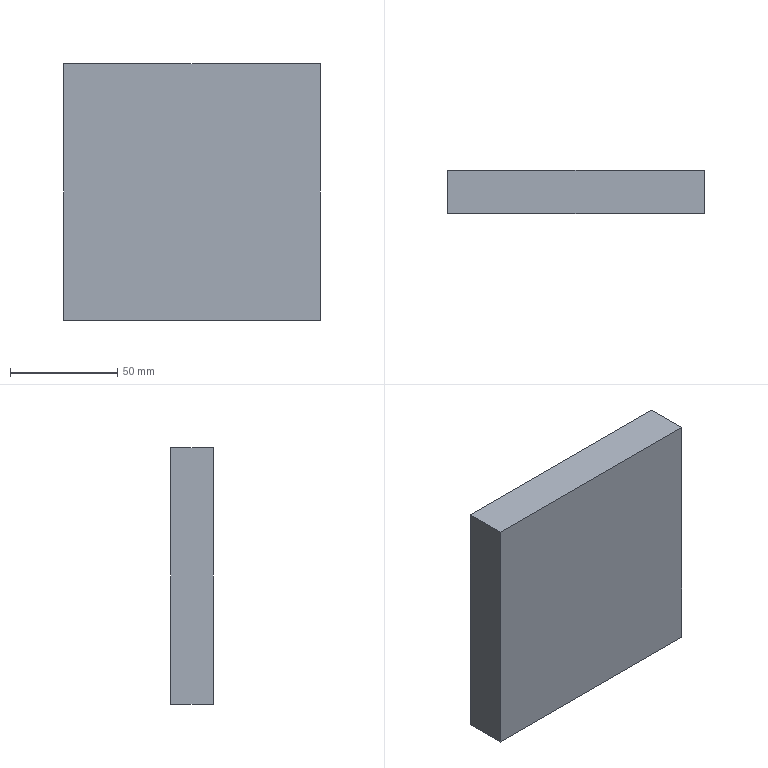Part | SolidWorks | features Extrusion 1 | 1 solid | 6 faces | box 120 x 20 x 120 mm | volume 288000 mm3 | plane 6
STEP:
#1=CARTESIAN_POINT('',(60.,0.,60.));
#2=VERTEX_POINT('',#1);
#3=CARTESIAN_POINT('',(60.,0.,-60.));
#4=VERTEX_POINT('',#3);
#5=CARTESIAN_POINT('',(60.,0.,-60.));
#6=DIRECTION('',(0.,0.,-1.));
#7=VECTOR('',#6,1000.);
#8=LINE('',#5,#7);
#9=EDGE_CURVE('',#2,#4,#8,.T.);
#10=ORIENTED_EDGE('',*,*,#9,.T.);
#11=CARTESIAN_POINT('',(60.,20.,-60.));
#12=VERTEX_POINT('',#11);
#13=CARTESIAN_POINT('',(60.,20.,-60.));
#14=DIRECTION('',(0.,-1.,0.));
#15=VECTOR('',#14,1000.);
#16=LINE('',#13,#15);
#17=EDGE_CURVE('',#12,#4,#16,.T.);
#18=ORIENTED_EDGE('',*,*,#17,.F.);
#19=CARTESIAN_POINT('',(60.,20.,60.));
#20=VERTEX_POINT('',#19);
#21=CARTESIAN_POINT('',(60.,20.,-60.));
#22=DIRECTION('',(0.,0.,-1.));
#23=VECTOR('',#22,1000.);
#24=LINE('',#21,#23);
#25=EDGE_CURVE('',#20,#12,#24,.T.);
#26=ORIENTED_EDGE('',*,*,#25,.F.);
#27=CARTESIAN_POINT('',(60.,20.,60.));
#28=DIRECTION('',(0.,-1.,0.));
#29=VECTOR('',#28,1000.);
#30=LINE('',#27,#29);
#31=EDGE_CURVE('',#20,#2,#30,.T.);
#32=ORIENTED_EDGE('',*,*,#31,.T.);
#33=EDGE_LOOP('',(#10,#18,#26,#32));
#34=FACE_OUTER_BOUND('',#33,.T.);
#35=CARTESIAN_POINT('',(60.,20.,-60.));
#36=DIRECTION('',(-1.,0.,0.));
#37=DIRECTION('',(0.,0.,1.));
#38=AXIS2_PLACEMENT_3D('',#35,#36,#37);
#39=PLANE('',#38);
#40=ADVANCED_FACE('',(#34),#39,.F.);
#41=CARTESIAN_POINT('',(-60.,0.,-60.));
#42=VERTEX_POINT('',#41);
#43=CARTESIAN_POINT('',(-60.,0.,-60.));
#44=DIRECTION('',(-1.,0.,0.));
#45=VECTOR('',#44,1000.);
#46=LINE('',#43,#45);
#47=EDGE_CURVE('',#4,#42,#46,.T.);
#48=ORIENTED_EDGE('',*,*,#47,.T.);
#49=CARTESIAN_POINT('',(-60.,20.,-60.));
#50=VERTEX_POINT('',#49);
#51=CARTESIAN_POINT('',(-60.,20.,-60.));
#52=DIRECTION('',(0.,-1.,0.));
#53=VECTOR('',#52,1000.);
#54=LINE('',#51,#53);
#55=EDGE_CURVE('',#50,#42,#54,.T.);
#56=ORIENTED_EDGE('',*,*,#55,.F.);
#57=CARTESIAN_POINT('',(-60.,20.,-60.));
#58=DIRECTION('',(-1.,0.,0.));
#59=VECTOR('',#58,1000.);
#60=LINE('',#57,#59);
#61=EDGE_CURVE('',#12,#50,#60,.T.);
#62=ORIENTED_EDGE('',*,*,#61,.F.);
#63=ORIENTED_EDGE('',*,*,#17,.T.);
#64=EDGE_LOOP('',(#48,#56,#62,#63));
#65=FACE_OUTER_BOUND('',#64,.T.);
#66=CARTESIAN_POINT('',(-60.,20.,-60.));
#67=DIRECTION('',(0.,0.,1.));
#68=DIRECTION('',(1.,0.,0.));
#69=AXIS2_PLACEMENT_3D('',#66,#67,#68);
#70=PLANE('',#69);
#71=ADVANCED_FACE('',(#65),#70,.F.);
#72=CARTESIAN_POINT('',(-60.,0.,60.));
#73=VERTEX_POINT('',#72);
#74=CARTESIAN_POINT('',(-60.,0.,-60.));
#75=DIRECTION('',(0.,0.,1.));
#76=VECTOR('',#75,1000.);
#77=LINE('',#74,#76);
#78=EDGE_CURVE('',#42,#73,#77,.T.);
#79=ORIENTED_EDGE('',*,*,#78,.T.);
#80=CARTESIAN_POINT('',(-60.,20.,60.));
#81=VERTEX_POINT('',#80);
#82=CARTESIAN_POINT('',(-60.,20.,60.));
#83=DIRECTION('',(0.,-1.,0.));
#84=VECTOR('',#83,1000.);
#85=LINE('',#82,#84);
#86=EDGE_CURVE('',#81,#73,#85,.T.);
#87=ORIENTED_EDGE('',*,*,#86,.F.);
#88=CARTESIAN_POINT('',(-60.,20.,-60.));
#89=DIRECTION('',(0.,0.,1.));
#90=VECTOR('',#89,1000.);
#91=LINE('',#88,#90);
#92=EDGE_CURVE('',#50,#81,#91,.T.);
#93=ORIENTED_EDGE('',*,*,#92,.F.);
#94=ORIENTED_EDGE('',*,*,#55,.T.);
#95=EDGE_LOOP('',(#79,#87,#93,#94));
#96=FACE_OUTER_BOUND('',#95,.T.);
#97=CARTESIAN_POINT('',(-60.,20.,-60.));
#98=DIRECTION('',(1.,0.,0.));
#99=DIRECTION('',(0.,0.,-1.));
#100=AXIS2_PLACEMENT_3D('',#97,#98,#99);
#101=PLANE('',#100);
#102=ADVANCED_FACE('',(#96),#101,.F.);
#103=CARTESIAN_POINT('',(-60.,0.,60.));
#104=DIRECTION('',(1.,0.,0.));
#105=VECTOR('',#104,1000.);
#106=LINE('',#103,#105);
#107=EDGE_CURVE('',#73,#2,#106,.T.);
#108=ORIENTED_EDGE('',*,*,#107,.T.);
#109=ORIENTED_EDGE('',*,*,#31,.F.);
#110=CARTESIAN_POINT('',(-60.,20.,60.));
#111=DIRECTION('',(1.,0.,0.));
#112=VECTOR('',#111,1000.);
#113=LINE('',#110,#112);
#114=EDGE_CURVE('',#81,#20,#113,.T.);
#115=ORIENTED_EDGE('',*,*,#114,.F.);
#116=ORIENTED_EDGE('',*,*,#86,.T.);
#117=EDGE_LOOP('',(#108,#109,#115,#116));
#118=FACE_OUTER_BOUND('',#117,.T.);
#119=CARTESIAN_POINT('',(-60.,20.,60.));
#120=DIRECTION('',(0.,0.,-1.));
#121=DIRECTION('',(-1.,0.,0.));
#122=AXIS2_PLACEMENT_3D('',#119,#120,#121);
#123=PLANE('',#122);
#124=ADVANCED_FACE('',(#118),#123,.F.);
#125=ORIENTED_EDGE('',*,*,#25,.T.);
#126=ORIENTED_EDGE('',*,*,#61,.T.);
#127=ORIENTED_EDGE('',*,*,#92,.T.);
#128=ORIENTED_EDGE('',*,*,#114,.T.);
#129=EDGE_LOOP('',(#125,#126,#127,#128));
#130=FACE_OUTER_BOUND('',#129,.T.);
#131=CARTESIAN_POINT('',(0.,20.,0.));
#132=DIRECTION('',(0.,1.,0.));
#133=DIRECTION('',(0.,0.,1.));
#134=AXIS2_PLACEMENT_3D('',#131,#132,#133);
#135=PLANE('',#134);
#136=ADVANCED_FACE('',(#130),#135,.T.);
#137=ORIENTED_EDGE('',*,*,#9,.F.);
#138=ORIENTED_EDGE('',*,*,#107,.F.);
#139=ORIENTED_EDGE('',*,*,#78,.F.);
#140=ORIENTED_EDGE('',*,*,#47,.F.);
#141=EDGE_LOOP('',(#137,#138,#139,#140));
#142=FACE_OUTER_BOUND('',#141,.T.);
#143=CARTESIAN_POINT('',(0.,0.,0.));
#144=DIRECTION('',(0.,1.,0.));
#145=DIRECTION('',(0.,0.,1.));
#146=AXIS2_PLACEMENT_3D('',#143,#144,#145);
#147=PLANE('',#146);
#148=ADVANCED_FACE('',(#142),#147,.F.);
#149=CLOSED_SHELL('',(#40,#71,#102,#124,#136,#148));
#150=MANIFOLD_SOLID_BREP('',#149);
#151=CARTESIAN_POINT('',(0.,0.,0.));
#152=DIRECTION('',(0.,0.,1.));
#153=DIRECTION('',(1.,0.,0.));
#154=AXIS2_PLACEMENT_3D('',#151,#152,#153);
#155=(LENGTH_UNIT()NAMED_UNIT(*)SI_UNIT(.MILLI.,.METRE.));
#156=UNCERTAINTY_MEASURE_WITH_UNIT(LENGTH_MEASURE(0.00001),#155,'','');
#157=(NAMED_UNIT(*)PLANE_ANGLE_UNIT()SI_UNIT($,.RADIAN.));
#158=(NAMED_UNIT(*)SI_UNIT($,.STERADIAN.)SOLID_ANGLE_UNIT());
#159=(GEOMETRIC_REPRESENTATION_CONTEXT(3)GLOBAL_UNCERTAINTY_ASSIGNED_CONTEXT((#156))GLOBAL_UNIT_ASSIGNED_CONTEXT((#155,#157,#158))REPRESENTATION_CONTEXT('',''));
#160=ADVANCED_BREP_SHAPE_REPRESENTATION('',(#150,#154),#159);